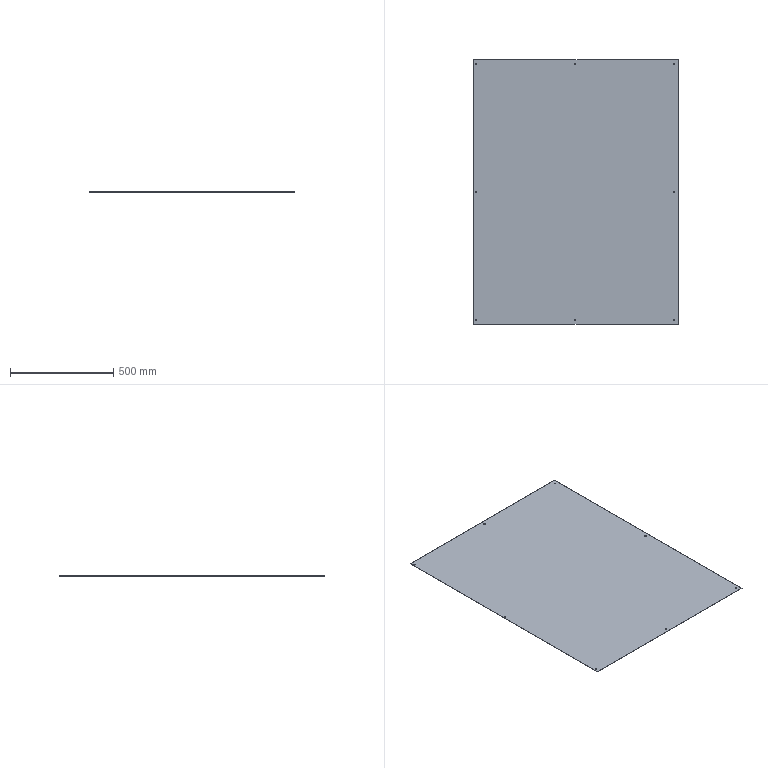Part | SolidWorks | features FlatPattern 1, HoleWzd 1, SMBaseFlange 1, SheetMetal 1 | 1 solid | 22 faces | box 990 x 1280 x 1.2 mm | volume 1520312 mm3 | cylinder 16 | plane 6 | commonest cylinder face diameters 6.6 x16
STEP:
#1=CARTESIAN_POINT('',(-488.3,620.,-1.2));
#2=VERTEX_POINT('',#1);
#3=CARTESIAN_POINT('',(-481.7,620.,-1.2));
#4=VERTEX_POINT('',#3);
#5=CARTESIAN_POINT('',(-485.,620.,-1.2));
#6=DIRECTION('',(0.,0.,1.));
#7=DIRECTION('',(1.,0.,0.));
#8=AXIS2_PLACEMENT_3D('',#5,#6,#7);
#9=CIRCLE('',#8,3.3);
#10=EDGE_CURVE('',#2,#4,#9,.T.);
#11=ORIENTED_EDGE('',*,*,#10,.F.);
#12=CARTESIAN_POINT('',(-488.3,620.,0.));
#13=VERTEX_POINT('',#12);
#14=CARTESIAN_POINT('',(-488.3,620.,0.));
#15=DIRECTION('',(0.,0.,1.));
#16=VECTOR('',#15,1000.);
#17=LINE('',#14,#16);
#18=EDGE_CURVE('',#2,#13,#17,.T.);
#19=ORIENTED_EDGE('',*,*,#18,.T.);
#20=CARTESIAN_POINT('',(-481.7,620.,0.));
#21=VERTEX_POINT('',#20);
#22=CARTESIAN_POINT('',(-485.,620.,0.));
#23=DIRECTION('',(0.,0.,1.));
#24=DIRECTION('',(1.,0.,0.));
#25=AXIS2_PLACEMENT_3D('',#22,#23,#24);
#26=CIRCLE('',#25,3.3);
#27=EDGE_CURVE('',#13,#21,#26,.T.);
#28=ORIENTED_EDGE('',*,*,#27,.T.);
#29=CARTESIAN_POINT('',(-481.7,620.,0.));
#30=DIRECTION('',(0.,0.,1.));
#31=VECTOR('',#30,1000.);
#32=LINE('',#29,#31);
#33=EDGE_CURVE('',#4,#21,#32,.T.);
#34=ORIENTED_EDGE('',*,*,#33,.F.);
#35=EDGE_LOOP('',(#11,#19,#28,#34));
#36=FACE_OUTER_BOUND('',#35,.T.);
#37=CARTESIAN_POINT('',(-485.,620.,0.));
#38=DIRECTION('',(0.,0.,1.));
#39=DIRECTION('',(1.,0.,0.));
#40=AXIS2_PLACEMENT_3D('',#37,#38,#39);
#41=CYLINDRICAL_SURFACE('',#40,3.3);
#42=ADVANCED_FACE('',(#36),#41,.F.);
#43=CARTESIAN_POINT('',(-8.3,620.,-1.2));
#44=VERTEX_POINT('',#43);
#45=CARTESIAN_POINT('',(-1.7,620.,-1.2));
#46=VERTEX_POINT('',#45);
#47=CARTESIAN_POINT('',(-5.,620.,-1.2));
#48=DIRECTION('',(0.,0.,1.));
#49=DIRECTION('',(1.,0.,0.));
#50=AXIS2_PLACEMENT_3D('',#47,#48,#49);
#51=CIRCLE('',#50,3.3);
#52=EDGE_CURVE('',#44,#46,#51,.T.);
#53=ORIENTED_EDGE('',*,*,#52,.F.);
#54=CARTESIAN_POINT('',(-8.3,620.,0.));
#55=VERTEX_POINT('',#54);
#56=CARTESIAN_POINT('',(-8.3,620.,0.));
#57=DIRECTION('',(0.,0.,1.));
#58=VECTOR('',#57,1000.);
#59=LINE('',#56,#58);
#60=EDGE_CURVE('',#44,#55,#59,.T.);
#61=ORIENTED_EDGE('',*,*,#60,.T.);
#62=CARTESIAN_POINT('',(-1.7,620.,0.));
#63=VERTEX_POINT('',#62);
#64=CARTESIAN_POINT('',(-5.,620.,0.));
#65=DIRECTION('',(0.,0.,1.));
#66=DIRECTION('',(1.,0.,0.));
#67=AXIS2_PLACEMENT_3D('',#64,#65,#66);
#68=CIRCLE('',#67,3.3);
#69=EDGE_CURVE('',#55,#63,#68,.T.);
#70=ORIENTED_EDGE('',*,*,#69,.T.);
#71=CARTESIAN_POINT('',(-1.7,620.,0.));
#72=DIRECTION('',(0.,0.,1.));
#73=VECTOR('',#72,1000.);
#74=LINE('',#71,#73);
#75=EDGE_CURVE('',#46,#63,#74,.T.);
#76=ORIENTED_EDGE('',*,*,#75,.F.);
#77=EDGE_LOOP('',(#53,#61,#70,#76));
#78=FACE_OUTER_BOUND('',#77,.T.);
#79=CARTESIAN_POINT('',(-5.,620.,0.));
#80=DIRECTION('',(0.,0.,1.));
#81=DIRECTION('',(1.,0.,0.));
#82=AXIS2_PLACEMENT_3D('',#79,#80,#81);
#83=CYLINDRICAL_SURFACE('',#82,3.3);
#84=ADVANCED_FACE('',(#78),#83,.F.);
#85=CARTESIAN_POINT('',(471.7,620.,-1.2));
#86=VERTEX_POINT('',#85);
#87=CARTESIAN_POINT('',(478.3,620.,-1.2));
#88=VERTEX_POINT('',#87);
#89=CARTESIAN_POINT('',(475.,620.,-1.2));
#90=DIRECTION('',(0.,0.,1.));
#91=DIRECTION('',(1.,0.,0.));
#92=AXIS2_PLACEMENT_3D('',#89,#90,#91);
#93=CIRCLE('',#92,3.3);
#94=EDGE_CURVE('',#86,#88,#93,.T.);
#95=ORIENTED_EDGE('',*,*,#94,.F.);
#96=CARTESIAN_POINT('',(471.7,620.,0.));
#97=VERTEX_POINT('',#96);
#98=CARTESIAN_POINT('',(471.7,620.,0.));
#99=DIRECTION('',(0.,0.,1.));
#100=VECTOR('',#99,1000.);
#101=LINE('',#98,#100);
#102=EDGE_CURVE('',#86,#97,#101,.T.);
#103=ORIENTED_EDGE('',*,*,#102,.T.);
#104=CARTESIAN_POINT('',(478.3,620.,0.));
#105=VERTEX_POINT('',#104);
#106=CARTESIAN_POINT('',(475.,620.,0.));
#107=DIRECTION('',(0.,0.,1.));
#108=DIRECTION('',(1.,0.,0.));
#109=AXIS2_PLACEMENT_3D('',#106,#107,#108);
#110=CIRCLE('',#109,3.3);
#111=EDGE_CURVE('',#97,#105,#110,.T.);
#112=ORIENTED_EDGE('',*,*,#111,.T.);
#113=CARTESIAN_POINT('',(478.3,620.,0.));
#114=DIRECTION('',(0.,0.,1.));
#115=VECTOR('',#114,1000.);
#116=LINE('',#113,#115);
#117=EDGE_CURVE('',#88,#105,#116,.T.);
#118=ORIENTED_EDGE('',*,*,#117,.F.);
#119=EDGE_LOOP('',(#95,#103,#112,#118));
#120=FACE_OUTER_BOUND('',#119,.T.);
#121=CARTESIAN_POINT('',(475.,620.,0.));
#122=DIRECTION('',(0.,0.,1.));
#123=DIRECTION('',(1.,0.,0.));
#124=AXIS2_PLACEMENT_3D('',#121,#122,#123);
#125=CYLINDRICAL_SURFACE('',#124,3.3);
#126=ADVANCED_FACE('',(#120),#125,.F.);
#127=CARTESIAN_POINT('',(471.7,0.,-1.2));
#128=VERTEX_POINT('',#127);
#129=CARTESIAN_POINT('',(478.3,0.,-1.2));
#130=VERTEX_POINT('',#129);
#131=CARTESIAN_POINT('',(475.,0.,-1.2));
#132=DIRECTION('',(0.,0.,1.));
#133=DIRECTION('',(1.,0.,0.));
#134=AXIS2_PLACEMENT_3D('',#131,#132,#133);
#135=CIRCLE('',#134,3.3);
#136=EDGE_CURVE('',#128,#130,#135,.T.);
#137=ORIENTED_EDGE('',*,*,#136,.F.);
#138=CARTESIAN_POINT('',(471.7,0.,0.));
#139=VERTEX_POINT('',#138);
#140=CARTESIAN_POINT('',(471.7,0.,0.));
#141=DIRECTION('',(0.,0.,1.));
#142=VECTOR('',#141,1000.);
#143=LINE('',#140,#142);
#144=EDGE_CURVE('',#128,#139,#143,.T.);
#145=ORIENTED_EDGE('',*,*,#144,.T.);
#146=CARTESIAN_POINT('',(478.3,0.,0.));
#147=VERTEX_POINT('',#146);
#148=CARTESIAN_POINT('',(475.,0.,0.));
#149=DIRECTION('',(0.,0.,1.));
#150=DIRECTION('',(1.,0.,0.));
#151=AXIS2_PLACEMENT_3D('',#148,#149,#150);
#152=CIRCLE('',#151,3.3);
#153=EDGE_CURVE('',#139,#147,#152,.T.);
#154=ORIENTED_EDGE('',*,*,#153,.T.);
#155=CARTESIAN_POINT('',(478.3,0.,0.));
#156=DIRECTION('',(0.,0.,1.));
#157=VECTOR('',#156,1000.);
#158=LINE('',#155,#157);
#159=EDGE_CURVE('',#130,#147,#158,.T.);
#160=ORIENTED_EDGE('',*,*,#159,.F.);
#161=EDGE_LOOP('',(#137,#145,#154,#160));
#162=FACE_OUTER_BOUND('',#161,.T.);
#163=CARTESIAN_POINT('',(475.,0.,0.));
#164=DIRECTION('',(0.,0.,1.));
#165=DIRECTION('',(1.,0.,0.));
#166=AXIS2_PLACEMENT_3D('',#163,#164,#165);
#167=CYLINDRICAL_SURFACE('',#166,3.3);
#168=ADVANCED_FACE('',(#162),#167,.F.);
#169=CARTESIAN_POINT('',(471.7,-620.,-1.2));
#170=VERTEX_POINT('',#169);
#171=CARTESIAN_POINT('',(478.3,-620.,-1.2));
#172=VERTEX_POINT('',#171);
#173=CARTESIAN_POINT('',(475.,-620.,-1.2));
#174=DIRECTION('',(0.,0.,1.));
#175=DIRECTION('',(1.,0.,0.));
#176=AXIS2_PLACEMENT_3D('',#173,#174,#175);
#177=CIRCLE('',#176,3.3);
#178=EDGE_CURVE('',#170,#172,#177,.T.);
#179=ORIENTED_EDGE('',*,*,#178,.F.);
#180=CARTESIAN_POINT('',(471.7,-620.,0.));
#181=VERTEX_POINT('',#180);
#182=CARTESIAN_POINT('',(471.7,-620.,0.));
#183=DIRECTION('',(0.,0.,1.));
#184=VECTOR('',#183,1000.);
#185=LINE('',#182,#184);
#186=EDGE_CURVE('',#170,#181,#185,.T.);
#187=ORIENTED_EDGE('',*,*,#186,.T.);
#188=CARTESIAN_POINT('',(478.3,-620.,0.));
#189=VERTEX_POINT('',#188);
#190=CARTESIAN_POINT('',(475.,-620.,0.));
#191=DIRECTION('',(0.,0.,1.));
#192=DIRECTION('',(1.,0.,0.));
#193=AXIS2_PLACEMENT_3D('',#190,#191,#192);
#194=CIRCLE('',#193,3.3);
#195=EDGE_CURVE('',#181,#189,#194,.T.);
#196=ORIENTED_EDGE('',*,*,#195,.T.);
#197=CARTESIAN_POINT('',(478.3,-620.,0.));
#198=DIRECTION('',(0.,0.,1.));
#199=VECTOR('',#198,1000.);
#200=LINE('',#197,#199);
#201=EDGE_CURVE('',#172,#189,#200,.T.);
#202=ORIENTED_EDGE('',*,*,#201,.F.);
#203=EDGE_LOOP('',(#179,#187,#196,#202));
#204=FACE_OUTER_BOUND('',#203,.T.);
#205=CARTESIAN_POINT('',(475.,-620.,0.));
#206=DIRECTION('',(0.,0.,1.));
#207=DIRECTION('',(1.,0.,0.));
#208=AXIS2_PLACEMENT_3D('',#205,#206,#207);
#209=CYLINDRICAL_SURFACE('',#208,3.3);
#210=ADVANCED_FACE('',(#204),#209,.F.);
#211=CARTESIAN_POINT('',(-8.3,-620.,-1.2));
#212=VERTEX_POINT('',#211);
#213=CARTESIAN_POINT('',(-1.7,-620.,-1.2));
#214=VERTEX_POINT('',#213);
#215=CARTESIAN_POINT('',(-5.,-620.,-1.2));
#216=DIRECTION('',(0.,0.,1.));
#217=DIRECTION('',(1.,0.,0.));
#218=AXIS2_PLACEMENT_3D('',#215,#216,#217);
#219=CIRCLE('',#218,3.3);
#220=EDGE_CURVE('',#212,#214,#219,.T.);
#221=ORIENTED_EDGE('',*,*,#220,.F.);
#222=CARTESIAN_POINT('',(-8.3,-620.,0.));
#223=VERTEX_POINT('',#222);
#224=CARTESIAN_POINT('',(-8.3,-620.,0.));
#225=DIRECTION('',(0.,0.,1.));
#226=VECTOR('',#225,1000.);
#227=LINE('',#224,#226);
#228=EDGE_CURVE('',#212,#223,#227,.T.);
#229=ORIENTED_EDGE('',*,*,#228,.T.);
#230=CARTESIAN_POINT('',(-1.7,-620.,0.));
#231=VERTEX_POINT('',#230);
#232=CARTESIAN_POINT('',(-5.,-620.,0.));
#233=DIRECTION('',(0.,0.,1.));
#234=DIRECTION('',(1.,0.,0.));
#235=AXIS2_PLACEMENT_3D('',#232,#233,#234);
#236=CIRCLE('',#235,3.3);
#237=EDGE_CURVE('',#223,#231,#236,.T.);
#238=ORIENTED_EDGE('',*,*,#237,.T.);
#239=CARTESIAN_POINT('',(-1.7,-620.,0.));
#240=DIRECTION('',(0.,0.,1.));
#241=VECTOR('',#240,1000.);
#242=LINE('',#239,#241);
#243=EDGE_CURVE('',#214,#231,#242,.T.);
#244=ORIENTED_EDGE('',*,*,#243,.F.);
#245=EDGE_LOOP('',(#221,#229,#238,#244));
#246=FACE_OUTER_BOUND('',#245,.T.);
#247=CARTESIAN_POINT('',(-5.,-620.,0.));
#248=DIRECTION('',(0.,0.,1.));
#249=DIRECTION('',(1.,0.,0.));
#250=AXIS2_PLACEMENT_3D('',#247,#248,#249);
#251=CYLINDRICAL_SURFACE('',#250,3.3);
#252=ADVANCED_FACE('',(#246),#251,.F.);
#253=CARTESIAN_POINT('',(-488.3,-620.,-1.2));
#254=VERTEX_POINT('',#253);
#255=CARTESIAN_POINT('',(-481.7,-620.,-1.2));
#256=VERTEX_POINT('',#255);
#257=CARTESIAN_POINT('',(-485.,-620.,-1.2));
#258=DIRECTION('',(0.,0.,1.));
#259=DIRECTION('',(1.,0.,0.));
#260=AXIS2_PLACEMENT_3D('',#257,#258,#259);
#261=CIRCLE('',#260,3.3);
#262=EDGE_CURVE('',#254,#256,#261,.T.);
#263=ORIENTED_EDGE('',*,*,#262,.F.);
#264=CARTESIAN_POINT('',(-488.3,-620.,0.));
#265=VERTEX_POINT('',#264);
#266=CARTESIAN_POINT('',(-488.3,-620.,0.));
#267=DIRECTION('',(0.,0.,1.));
#268=VECTOR('',#267,1000.);
#269=LINE('',#266,#268);
#270=EDGE_CURVE('',#254,#265,#269,.T.);
#271=ORIENTED_EDGE('',*,*,#270,.T.);
#272=CARTESIAN_POINT('',(-481.7,-620.,0.));
#273=VERTEX_POINT('',#272);
#274=CARTESIAN_POINT('',(-485.,-620.,0.));
#275=DIRECTION('',(0.,0.,1.));
#276=DIRECTION('',(1.,0.,0.));
#277=AXIS2_PLACEMENT_3D('',#274,#275,#276);
#278=CIRCLE('',#277,3.3);
#279=EDGE_CURVE('',#265,#273,#278,.T.);
#280=ORIENTED_EDGE('',*,*,#279,.T.);
#281=CARTESIAN_POINT('',(-481.7,-620.,0.));
#282=DIRECTION('',(0.,0.,1.));
#283=VECTOR('',#282,1000.);
#284=LINE('',#281,#283);
#285=EDGE_CURVE('',#256,#273,#284,.T.);
#286=ORIENTED_EDGE('',*,*,#285,.F.);
#287=EDGE_LOOP('',(#263,#271,#280,#286));
#288=FACE_OUTER_BOUND('',#287,.T.);
#289=CARTESIAN_POINT('',(-485.,-620.,0.));
#290=DIRECTION('',(0.,0.,1.));
#291=DIRECTION('',(1.,0.,0.));
#292=AXIS2_PLACEMENT_3D('',#289,#290,#291);
#293=CYLINDRICAL_SURFACE('',#292,3.3);
#294=ADVANCED_FACE('',(#288),#293,.F.);
#295=CARTESIAN_POINT('',(-488.3,0.,-1.2));
#296=VERTEX_POINT('',#295);
#297=CARTESIAN_POINT('',(-481.7,0.,-1.2));
#298=VERTEX_POINT('',#297);
#299=CARTESIAN_POINT('',(-485.,0.,-1.2));
#300=DIRECTION('',(0.,0.,1.));
#301=DIRECTION('',(1.,0.,0.));
#302=AXIS2_PLACEMENT_3D('',#299,#300,#301);
#303=CIRCLE('',#302,3.3);
#304=EDGE_CURVE('',#296,#298,#303,.T.);
#305=ORIENTED_EDGE('',*,*,#304,.F.);
#306=CARTESIAN_POINT('',(-488.3,0.,0.));
#307=VERTEX_POINT('',#306);
#308=CARTESIAN_POINT('',(-488.3,0.,0.));
#309=DIRECTION('',(0.,0.,1.));
#310=VECTOR('',#309,1000.);
#311=LINE('',#308,#310);
#312=EDGE_CURVE('',#296,#307,#311,.T.);
#313=ORIENTED_EDGE('',*,*,#312,.T.);
#314=CARTESIAN_POINT('',(-481.7,0.,0.));
#315=VERTEX_POINT('',#314);
#316=CARTESIAN_POINT('',(-485.,0.,0.));
#317=DIRECTION('',(0.,0.,1.));
#318=DIRECTION('',(1.,0.,0.));
#319=AXIS2_PLACEMENT_3D('',#316,#317,#318);
#320=CIRCLE('',#319,3.3);
#321=EDGE_CURVE('',#307,#315,#320,.T.);
#322=ORIENTED_EDGE('',*,*,#321,.T.);
#323=CARTESIAN_POINT('',(-481.7,0.,0.));
#324=DIRECTION('',(0.,0.,1.));
#325=VECTOR('',#324,1000.);
#326=LINE('',#323,#325);
#327=EDGE_CURVE('',#298,#315,#326,.T.);
#328=ORIENTED_EDGE('',*,*,#327,.F.);
#329=EDGE_LOOP('',(#305,#313,#322,#328));
#330=FACE_OUTER_BOUND('',#329,.T.);
#331=CARTESIAN_POINT('',(-485.,0.,0.));
#332=DIRECTION('',(0.,0.,1.));
#333=DIRECTION('',(1.,0.,0.));
#334=AXIS2_PLACEMENT_3D('',#331,#332,#333);
#335=CYLINDRICAL_SURFACE('',#334,3.3);
#336=ADVANCED_FACE('',(#330),#335,.F.);
#337=CARTESIAN_POINT('',(495.,-640.,0.));
#338=VERTEX_POINT('',#337);
#339=CARTESIAN_POINT('',(495.,640.,0.));
#340=VERTEX_POINT('',#339);
#341=CARTESIAN_POINT('',(495.,640.,0.));
#342=DIRECTION('',(0.,1.,0.));
#343=VECTOR('',#342,1000.);
#344=LINE('',#341,#343);
#345=EDGE_CURVE('',#338,#340,#344,.T.);
#346=ORIENTED_EDGE('',*,*,#345,.F.);
#347=CARTESIAN_POINT('',(495.,-640.,-1.2));
#348=VERTEX_POINT('',#347);
#349=CARTESIAN_POINT('',(495.,-640.,-1.2));
#350=DIRECTION('',(0.,0.,1.));
#351=VECTOR('',#350,1000.);
#352=LINE('',#349,#351);
#353=EDGE_CURVE('',#348,#338,#352,.T.);
#354=ORIENTED_EDGE('',*,*,#353,.F.);
#355=CARTESIAN_POINT('',(495.,640.,-1.2));
#356=VERTEX_POINT('',#355);
#357=CARTESIAN_POINT('',(495.,640.,-1.2));
#358=DIRECTION('',(0.,1.,0.));
#359=VECTOR('',#358,1000.);
#360=LINE('',#357,#359);
#361=EDGE_CURVE('',#348,#356,#360,.T.);
#362=ORIENTED_EDGE('',*,*,#361,.T.);
#363=CARTESIAN_POINT('',(495.,640.,-1.2));
#364=DIRECTION('',(0.,0.,1.));
#365=VECTOR('',#364,1000.);
#366=LINE('',#363,#365);
#367=EDGE_CURVE('',#356,#340,#366,.T.);
#368=ORIENTED_EDGE('',*,*,#367,.T.);
#369=EDGE_LOOP('',(#346,#354,#362,#368));
#370=FACE_OUTER_BOUND('',#369,.T.);
#371=CARTESIAN_POINT('',(495.,640.,-1.2));
#372=DIRECTION('',(1.,0.,0.));
#373=DIRECTION('',(0.,1.,0.));
#374=AXIS2_PLACEMENT_3D('',#371,#372,#373);
#375=PLANE('',#374);
#376=ADVANCED_FACE('',(#370),#375,.T.);
#377=CARTESIAN_POINT('',(-495.,-640.,0.));
#378=VERTEX_POINT('',#377);
#379=CARTESIAN_POINT('',(-495.,-640.,0.));
#380=DIRECTION('',(1.,0.,0.));
#381=VECTOR('',#380,1000.);
#382=LINE('',#379,#381);
#383=EDGE_CURVE('',#378,#338,#382,.T.);
#384=ORIENTED_EDGE('',*,*,#383,.F.);
#385=CARTESIAN_POINT('',(-495.,-640.,-1.2));
#386=VERTEX_POINT('',#385);
#387=CARTESIAN_POINT('',(-495.,-640.,-1.2));
#388=DIRECTION('',(0.,0.,1.));
#389=VECTOR('',#388,1000.);
#390=LINE('',#387,#389);
#391=EDGE_CURVE('',#386,#378,#390,.T.);
#392=ORIENTED_EDGE('',*,*,#391,.F.);
#393=CARTESIAN_POINT('',(-495.,-640.,-1.2));
#394=DIRECTION('',(1.,0.,0.));
#395=VECTOR('',#394,1000.);
#396=LINE('',#393,#395);
#397=EDGE_CURVE('',#386,#348,#396,.T.);
#398=ORIENTED_EDGE('',*,*,#397,.T.);
#399=ORIENTED_EDGE('',*,*,#353,.T.);
#400=EDGE_LOOP('',(#384,#392,#398,#399));
#401=FACE_OUTER_BOUND('',#400,.T.);
#402=CARTESIAN_POINT('',(-495.,-640.,-1.2));
#403=DIRECTION('',(0.,-1.,0.));
#404=DIRECTION('',(0.,0.,-1.));
#405=AXIS2_PLACEMENT_3D('',#402,#403,#404);
#406=PLANE('',#405);
#407=ADVANCED_FACE('',(#401),#406,.T.);
#408=CARTESIAN_POINT('',(-495.,640.,0.));
#409=VERTEX_POINT('',#408);
#410=CARTESIAN_POINT('',(-495.,640.,0.));
#411=DIRECTION('',(0.,-1.,0.));
#412=VECTOR('',#411,1000.);
#413=LINE('',#410,#412);
#414=EDGE_CURVE('',#409,#378,#413,.T.);
#415=ORIENTED_EDGE('',*,*,#414,.F.);
#416=CARTESIAN_POINT('',(-495.,640.,-1.2));
#417=VERTEX_POINT('',#416);
#418=CARTESIAN_POINT('',(-495.,640.,-1.2));
#419=DIRECTION('',(0.,0.,1.));
#420=VECTOR('',#419,1000.);
#421=LINE('',#418,#420);
#422=EDGE_CURVE('',#417,#409,#421,.T.);
#423=ORIENTED_EDGE('',*,*,#422,.F.);
#424=CARTESIAN_POINT('',(-495.,640.,-1.2));
#425=DIRECTION('',(0.,-1.,0.));
#426=VECTOR('',#425,1000.);
#427=LINE('',#424,#426);
#428=EDGE_CURVE('',#417,#386,#427,.T.);
#429=ORIENTED_EDGE('',*,*,#428,.T.);
#430=ORIENTED_EDGE('',*,*,#391,.T.);
#431=EDGE_LOOP('',(#415,#423,#429,#430));
#432=FACE_OUTER_BOUND('',#431,.T.);
#433=CARTESIAN_POINT('',(-495.,640.,-1.2));
#434=DIRECTION('',(-1.,0.,0.));
#435=DIRECTION('',(0.,-1.,0.));
#436=AXIS2_PLACEMENT_3D('',#433,#434,#435);
#437=PLANE('',#436);
#438=ADVANCED_FACE('',(#432),#437,.T.);
#439=CARTESIAN_POINT('',(-495.,640.,0.));
#440=DIRECTION('',(-1.,0.,0.));
#441=VECTOR('',#440,1000.);
#442=LINE('',#439,#441);
#443=EDGE_CURVE('',#340,#409,#442,.T.);
#444=ORIENTED_EDGE('',*,*,#443,.F.);
#445=ORIENTED_EDGE('',*,*,#367,.F.);
#446=CARTESIAN_POINT('',(-495.,640.,-1.2));
#447=DIRECTION('',(-1.,0.,0.));
#448=VECTOR('',#447,1000.);
#449=LINE('',#446,#448);
#450=EDGE_CURVE('',#356,#417,#449,.T.);
#451=ORIENTED_EDGE('',*,*,#450,.T.);
#452=ORIENTED_EDGE('',*,*,#422,.T.);
#453=EDGE_LOOP('',(#444,#445,#451,#452));
#454=FACE_OUTER_BOUND('',#453,.T.);
#455=CARTESIAN_POINT('',(-495.,640.,-1.2));
#456=DIRECTION('',(0.,1.,0.));
#457=DIRECTION('',(0.,0.,1.));
#458=AXIS2_PLACEMENT_3D('',#455,#456,#457);
#459=PLANE('',#458);
#460=ADVANCED_FACE('',(#454),#459,.T.);
#461=CARTESIAN_POINT('',(-485.,620.,-1.2));
#462=DIRECTION('',(0.,0.,1.));
#463=DIRECTION('',(1.,0.,0.));
#464=AXIS2_PLACEMENT_3D('',#461,#462,#463);
#465=CIRCLE('',#464,3.3);
#466=EDGE_CURVE('',#4,#2,#465,.T.);
#467=ORIENTED_EDGE('',*,*,#466,.T.);
#468=ORIENTED_EDGE('',*,*,#10,.T.);
#469=EDGE_LOOP('',(#467,#468));
#470=FACE_BOUND('',#469,.T.);
#471=CARTESIAN_POINT('',(-5.,620.,-1.2));
#472=DIRECTION('',(0.,0.,1.));
#473=DIRECTION('',(1.,0.,0.));
#474=AXIS2_PLACEMENT_3D('',#471,#472,#473);
#475=CIRCLE('',#474,3.3);
#476=EDGE_CURVE('',#46,#44,#475,.T.);
#477=ORIENTED_EDGE('',*,*,#476,.T.);
#478=ORIENTED_EDGE('',*,*,#52,.T.);
#479=EDGE_LOOP('',(#477,#478));
#480=FACE_BOUND('',#479,.T.);
#481=CARTESIAN_POINT('',(475.,620.,-1.2));
#482=DIRECTION('',(0.,0.,1.));
#483=DIRECTION('',(1.,0.,0.));
#484=AXIS2_PLACEMENT_3D('',#481,#482,#483);
#485=CIRCLE('',#484,3.3);
#486=EDGE_CURVE('',#88,#86,#485,.T.);
#487=ORIENTED_EDGE('',*,*,#486,.T.);
#488=ORIENTED_EDGE('',*,*,#94,.T.);
#489=EDGE_LOOP('',(#487,#488));
#490=FACE_BOUND('',#489,.T.);
#491=CARTESIAN_POINT('',(475.,0.,-1.2));
#492=DIRECTION('',(0.,0.,1.));
#493=DIRECTION('',(1.,0.,0.));
#494=AXIS2_PLACEMENT_3D('',#491,#492,#493);
#495=CIRCLE('',#494,3.3);
#496=EDGE_CURVE('',#130,#128,#495,.T.);
#497=ORIENTED_EDGE('',*,*,#496,.T.);
#498=ORIENTED_EDGE('',*,*,#136,.T.);
#499=EDGE_LOOP('',(#497,#498));
#500=FACE_BOUND('',#499,.T.);
#501=CARTESIAN_POINT('',(475.,-620.,-1.2));
#502=DIRECTION('',(0.,0.,1.));
#503=DIRECTION('',(1.,0.,0.));
#504=AXIS2_PLACEMENT_3D('',#501,#502,#503);
#505=CIRCLE('',#504,3.3);
#506=EDGE_CURVE('',#172,#170,#505,.T.);
#507=ORIENTED_EDGE('',*,*,#506,.T.);
#508=ORIENTED_EDGE('',*,*,#178,.T.);
#509=EDGE_LOOP('',(#507,#508));
#510=FACE_BOUND('',#509,.T.);
#511=CARTESIAN_POINT('',(-5.,-620.,-1.2));
#512=DIRECTION('',(0.,0.,1.));
#513=DIRECTION('',(1.,0.,0.));
#514=AXIS2_PLACEMENT_3D('',#511,#512,#513);
#515=CIRCLE('',#514,3.3);
#516=EDGE_CURVE('',#214,#212,#515,.T.);
#517=ORIENTED_EDGE('',*,*,#516,.T.);
#518=ORIENTED_EDGE('',*,*,#220,.T.);
#519=EDGE_LOOP('',(#517,#518));
#520=FACE_BOUND('',#519,.T.);
#521=CARTESIAN_POINT('',(-485.,-620.,-1.2));
#522=DIRECTION('',(0.,0.,1.));
#523=DIRECTION('',(1.,0.,0.));
#524=AXIS2_PLACEMENT_3D('',#521,#522,#523);
#525=CIRCLE('',#524,3.3);
#526=EDGE_CURVE('',#256,#254,#525,.T.);
#527=ORIENTED_EDGE('',*,*,#526,.T.);
#528=ORIENTED_EDGE('',*,*,#262,.T.);
#529=EDGE_LOOP('',(#527,#528));
#530=FACE_BOUND('',#529,.T.);
#531=CARTESIAN_POINT('',(-485.,0.,-1.2));
#532=DIRECTION('',(0.,0.,1.));
#533=DIRECTION('',(1.,0.,0.));
#534=AXIS2_PLACEMENT_3D('',#531,#532,#533);
#535=CIRCLE('',#534,3.3);
#536=EDGE_CURVE('',#298,#296,#535,.T.);
#537=ORIENTED_EDGE('',*,*,#536,.T.);
#538=ORIENTED_EDGE('',*,*,#304,.T.);
#539=EDGE_LOOP('',(#537,#538));
#540=FACE_BOUND('',#539,.T.);
#541=ORIENTED_EDGE('',*,*,#361,.F.);
#542=ORIENTED_EDGE('',*,*,#397,.F.);
#543=ORIENTED_EDGE('',*,*,#428,.F.);
#544=ORIENTED_EDGE('',*,*,#450,.F.);
#545=EDGE_LOOP('',(#541,#542,#543,#544));
#546=FACE_OUTER_BOUND('',#545,.T.);
#547=CARTESIAN_POINT('',(0.,0.,-1.2));
#548=DIRECTION('',(0.,0.,1.));
#549=DIRECTION('',(1.,0.,0.));
#550=AXIS2_PLACEMENT_3D('',#547,#548,#549);
#551=PLANE('',#550);
#552=ADVANCED_FACE('',(#470,#480,#490,#500,#510,#520,#530,#540,#546),#551,.F.);
#553=CARTESIAN_POINT('',(-485.,620.,0.));
#554=DIRECTION('',(0.,0.,1.));
#555=DIRECTION('',(1.,0.,0.));
#556=AXIS2_PLACEMENT_3D('',#553,#554,#555);
#557=CIRCLE('',#556,3.3);
#558=EDGE_CURVE('',#21,#13,#557,.T.);
#559=ORIENTED_EDGE('',*,*,#558,.F.);
#560=ORIENTED_EDGE('',*,*,#27,.F.);
#561=EDGE_LOOP('',(#559,#560));
#562=FACE_BOUND('',#561,.T.);
#563=CARTESIAN_POINT('',(-5.,620.,0.));
#564=DIRECTION('',(0.,0.,1.));
#565=DIRECTION('',(1.,0.,0.));
#566=AXIS2_PLACEMENT_3D('',#563,#564,#565);
#567=CIRCLE('',#566,3.3);
#568=EDGE_CURVE('',#63,#55,#567,.T.);
#569=ORIENTED_EDGE('',*,*,#568,.F.);
#570=ORIENTED_EDGE('',*,*,#69,.F.);
#571=EDGE_LOOP('',(#569,#570));
#572=FACE_BOUND('',#571,.T.);
#573=CARTESIAN_POINT('',(475.,620.,0.));
#574=DIRECTION('',(0.,0.,1.));
#575=DIRECTION('',(1.,0.,0.));
#576=AXIS2_PLACEMENT_3D('',#573,#574,#575);
#577=CIRCLE('',#576,3.3);
#578=EDGE_CURVE('',#105,#97,#577,.T.);
#579=ORIENTED_EDGE('',*,*,#578,.F.);
#580=ORIENTED_EDGE('',*,*,#111,.F.);
#581=EDGE_LOOP('',(#579,#580));
#582=FACE_BOUND('',#581,.T.);
#583=CARTESIAN_POINT('',(475.,0.,0.));
#584=DIRECTION('',(0.,0.,1.));
#585=DIRECTION('',(1.,0.,0.));
#586=AXIS2_PLACEMENT_3D('',#583,#584,#585);
#587=CIRCLE('',#586,3.3);
#588=EDGE_CURVE('',#147,#139,#587,.T.);
#589=ORIENTED_EDGE('',*,*,#588,.F.);
#590=ORIENTED_EDGE('',*,*,#153,.F.);
#591=EDGE_LOOP('',(#589,#590));
#592=FACE_BOUND('',#591,.T.);
#593=CARTESIAN_POINT('',(475.,-620.,0.));
#594=DIRECTION('',(0.,0.,1.));
#595=DIRECTION('',(1.,0.,0.));
#596=AXIS2_PLACEMENT_3D('',#593,#594,#595);
#597=CIRCLE('',#596,3.3);
#598=EDGE_CURVE('',#189,#181,#597,.T.);
#599=ORIENTED_EDGE('',*,*,#598,.F.);
#600=ORIENTED_EDGE('',*,*,#195,.F.);
#601=EDGE_LOOP('',(#599,#600));
#602=FACE_BOUND('',#601,.T.);
#603=CARTESIAN_POINT('',(-5.,-620.,0.));
#604=DIRECTION('',(0.,0.,1.));
#605=DIRECTION('',(1.,0.,0.));
#606=AXIS2_PLACEMENT_3D('',#603,#604,#605);
#607=CIRCLE('',#606,3.3);
#608=EDGE_CURVE('',#231,#223,#607,.T.);
#609=ORIENTED_EDGE('',*,*,#608,.F.);
#610=ORIENTED_EDGE('',*,*,#237,.F.);
#611=EDGE_LOOP('',(#609,#610));
#612=FACE_BOUND('',#611,.T.);
#613=CARTESIAN_POINT('',(-485.,-620.,0.));
#614=DIRECTION('',(0.,0.,1.));
#615=DIRECTION('',(1.,0.,0.));
#616=AXIS2_PLACEMENT_3D('',#613,#614,#615);
#617=CIRCLE('',#616,3.3);
#618=EDGE_CURVE('',#273,#265,#617,.T.);
#619=ORIENTED_EDGE('',*,*,#618,.F.);
#620=ORIENTED_EDGE('',*,*,#279,.F.);
#621=EDGE_LOOP('',(#619,#620));
#622=FACE_BOUND('',#621,.T.);
#623=CARTESIAN_POINT('',(-485.,0.,0.));
#624=DIRECTION('',(0.,0.,1.));
#625=DIRECTION('',(1.,0.,0.));
#626=AXIS2_PLACEMENT_3D('',#623,#624,#625);
#627=CIRCLE('',#626,3.3);
#628=EDGE_CURVE('',#315,#307,#627,.T.);
#629=ORIENTED_EDGE('',*,*,#628,.F.);
#630=ORIENTED_EDGE('',*,*,#321,.F.);
#631=EDGE_LOOP('',(#629,#630));
#632=FACE_BOUND('',#631,.T.);
#633=ORIENTED_EDGE('',*,*,#345,.T.);
#634=ORIENTED_EDGE('',*,*,#443,.T.);
#635=ORIENTED_EDGE('',*,*,#414,.T.);
#636=ORIENTED_EDGE('',*,*,#383,.T.);
#637=EDGE_LOOP('',(#633,#634,#635,#636));
#638=FACE_OUTER_BOUND('',#637,.T.);
#639=CARTESIAN_POINT('',(0.,0.,0.));
#640=DIRECTION('',(0.,0.,1.));
#641=DIRECTION('',(1.,0.,0.));
#642=AXIS2_PLACEMENT_3D('',#639,#640,#641);
#643=PLANE('',#642);
#644=ADVANCED_FACE('',(#562,#572,#582,#592,#602,#612,#622,#632,#638),#643,.T.);
#645=ORIENTED_EDGE('',*,*,#312,.F.);
#646=ORIENTED_EDGE('',*,*,#536,.F.);
#647=ORIENTED_EDGE('',*,*,#327,.T.);
#648=ORIENTED_EDGE('',*,*,#628,.T.);
#649=EDGE_LOOP('',(#645,#646,#647,#648));
#650=FACE_OUTER_BOUND('',#649,.T.);
#651=CARTESIAN_POINT('',(-485.,0.,0.));
#652=DIRECTION('',(0.,0.,1.));
#653=DIRECTION('',(1.,0.,0.));
#654=AXIS2_PLACEMENT_3D('',#651,#652,#653);
#655=CYLINDRICAL_SURFACE('',#654,3.3);
#656=ADVANCED_FACE('',(#650),#655,.F.);
#657=ORIENTED_EDGE('',*,*,#270,.F.);
#658=ORIENTED_EDGE('',*,*,#526,.F.);
#659=ORIENTED_EDGE('',*,*,#285,.T.);
#660=ORIENTED_EDGE('',*,*,#618,.T.);
#661=EDGE_LOOP('',(#657,#658,#659,#660));
#662=FACE_OUTER_BOUND('',#661,.T.);
#663=CARTESIAN_POINT('',(-485.,-620.,0.));
#664=DIRECTION('',(0.,0.,1.));
#665=DIRECTION('',(1.,0.,0.));
#666=AXIS2_PLACEMENT_3D('',#663,#664,#665);
#667=CYLINDRICAL_SURFACE('',#666,3.3);
#668=ADVANCED_FACE('',(#662),#667,.F.);
#669=ORIENTED_EDGE('',*,*,#228,.F.);
#670=ORIENTED_EDGE('',*,*,#516,.F.);
#671=ORIENTED_EDGE('',*,*,#243,.T.);
#672=ORIENTED_EDGE('',*,*,#608,.T.);
#673=EDGE_LOOP('',(#669,#670,#671,#672));
#674=FACE_OUTER_BOUND('',#673,.T.);
#675=CARTESIAN_POINT('',(-5.,-620.,0.));
#676=DIRECTION('',(0.,0.,1.));
#677=DIRECTION('',(1.,0.,0.));
#678=AXIS2_PLACEMENT_3D('',#675,#676,#677);
#679=CYLINDRICAL_SURFACE('',#678,3.3);
#680=ADVANCED_FACE('',(#674),#679,.F.);
#681=ORIENTED_EDGE('',*,*,#186,.F.);
#682=ORIENTED_EDGE('',*,*,#506,.F.);
#683=ORIENTED_EDGE('',*,*,#201,.T.);
#684=ORIENTED_EDGE('',*,*,#598,.T.);
#685=EDGE_LOOP('',(#681,#682,#683,#684));
#686=FACE_OUTER_BOUND('',#685,.T.);
#687=CARTESIAN_POINT('',(475.,-620.,0.));
#688=DIRECTION('',(0.,0.,1.));
#689=DIRECTION('',(1.,0.,0.));
#690=AXIS2_PLACEMENT_3D('',#687,#688,#689);
#691=CYLINDRICAL_SURFACE('',#690,3.3);
#692=ADVANCED_FACE('',(#686),#691,.F.);
#693=ORIENTED_EDGE('',*,*,#144,.F.);
#694=ORIENTED_EDGE('',*,*,#496,.F.);
#695=ORIENTED_EDGE('',*,*,#159,.T.);
#696=ORIENTED_EDGE('',*,*,#588,.T.);
#697=EDGE_LOOP('',(#693,#694,#695,#696));
#698=FACE_OUTER_BOUND('',#697,.T.);
#699=CARTESIAN_POINT('',(475.,0.,0.));
#700=DIRECTION('',(0.,0.,1.));
#701=DIRECTION('',(1.,0.,0.));
#702=AXIS2_PLACEMENT_3D('',#699,#700,#701);
#703=CYLINDRICAL_SURFACE('',#702,3.3);
#704=ADVANCED_FACE('',(#698),#703,.F.);
#705=ORIENTED_EDGE('',*,*,#102,.F.);
#706=ORIENTED_EDGE('',*,*,#486,.F.);
#707=ORIENTED_EDGE('',*,*,#117,.T.);
#708=ORIENTED_EDGE('',*,*,#578,.T.);
#709=EDGE_LOOP('',(#705,#706,#707,#708));
#710=FACE_OUTER_BOUND('',#709,.T.);
#711=CARTESIAN_POINT('',(475.,620.,0.));
#712=DIRECTION('',(0.,0.,1.));
#713=DIRECTION('',(1.,0.,0.));
#714=AXIS2_PLACEMENT_3D('',#711,#712,#713);
#715=CYLINDRICAL_SURFACE('',#714,3.3);
#716=ADVANCED_FACE('',(#710),#715,.F.);
#717=ORIENTED_EDGE('',*,*,#60,.F.);
#718=ORIENTED_EDGE('',*,*,#476,.F.);
#719=ORIENTED_EDGE('',*,*,#75,.T.);
#720=ORIENTED_EDGE('',*,*,#568,.T.);
#721=EDGE_LOOP('',(#717,#718,#719,#720));
#722=FACE_OUTER_BOUND('',#721,.T.);
#723=CARTESIAN_POINT('',(-5.,620.,0.));
#724=DIRECTION('',(0.,0.,1.));
#725=DIRECTION('',(1.,0.,0.));
#726=AXIS2_PLACEMENT_3D('',#723,#724,#725);
#727=CYLINDRICAL_SURFACE('',#726,3.3);
#728=ADVANCED_FACE('',(#722),#727,.F.);
#729=ORIENTED_EDGE('',*,*,#18,.F.);
#730=ORIENTED_EDGE('',*,*,#466,.F.);
#731=ORIENTED_EDGE('',*,*,#33,.T.);
#732=ORIENTED_EDGE('',*,*,#558,.T.);
#733=EDGE_LOOP('',(#729,#730,#731,#732));
#734=FACE_OUTER_BOUND('',#733,.T.);
#735=CARTESIAN_POINT('',(-485.,620.,0.));
#736=DIRECTION('',(0.,0.,1.));
#737=DIRECTION('',(1.,0.,0.));
#738=AXIS2_PLACEMENT_3D('',#735,#736,#737);
#739=CYLINDRICAL_SURFACE('',#738,3.3);
#740=ADVANCED_FACE('',(#734),#739,.F.);
#741=CLOSED_SHELL('',(#42,#84,#126,#168,#210,#252,#294,#336,#376,#407,#438,#460,#552,#644,#656,#668,#680,#692,#704,#716,#728,#740));
#742=MANIFOLD_SOLID_BREP('',#741);
#743=CARTESIAN_POINT('',(0.,0.,0.));
#744=DIRECTION('',(0.,0.,1.));
#745=DIRECTION('',(1.,0.,0.));
#746=AXIS2_PLACEMENT_3D('',#743,#744,#745);
#747=(LENGTH_UNIT()NAMED_UNIT(*)SI_UNIT(.MILLI.,.METRE.));
#748=UNCERTAINTY_MEASURE_WITH_UNIT(LENGTH_MEASURE(0.00001),#747,'','');
#749=(NAMED_UNIT(*)PLANE_ANGLE_UNIT()SI_UNIT($,.RADIAN.));
#750=(NAMED_UNIT(*)SI_UNIT($,.STERADIAN.)SOLID_ANGLE_UNIT());
#751=(GEOMETRIC_REPRESENTATION_CONTEXT(3)GLOBAL_UNCERTAINTY_ASSIGNED_CONTEXT((#748))GLOBAL_UNIT_ASSIGNED_CONTEXT((#747,#749,#750))REPRESENTATION_CONTEXT('',''));
#752=ADVANCED_BREP_SHAPE_REPRESENTATION('',(#742,#746),#751);